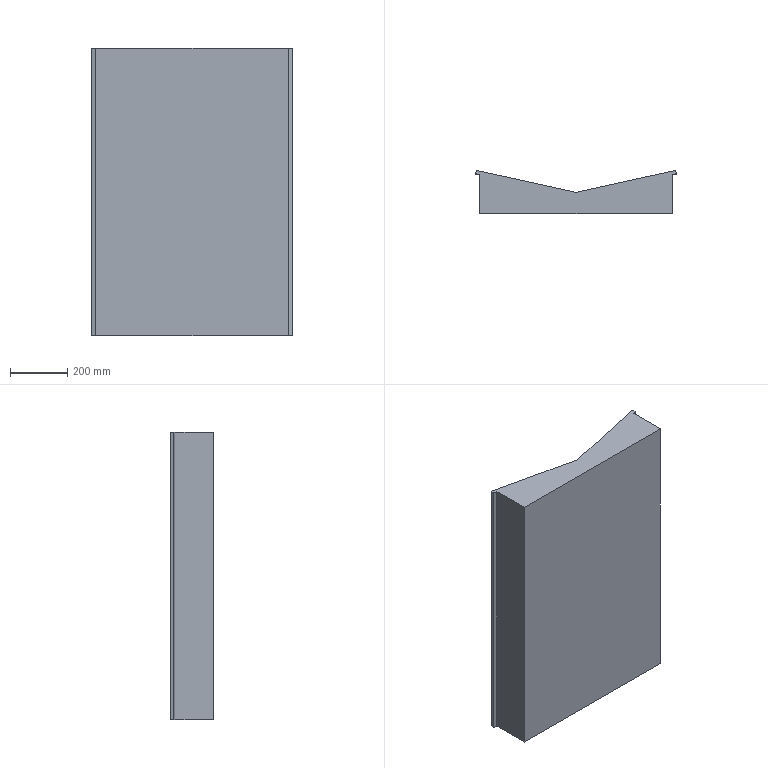Part | SolidWorks | features BaseBody 1 | 1 solid | 12 faces | box 698.157 x 148.827 x 1000 mm | volume 73538698 mm3 | plane 12
STEP:
#1=CARTESIAN_POINT('',(3335.082,1662.192,0.));
#2=VERTEX_POINT('',#1);
#3=CARTESIAN_POINT('',(3335.082,1796.192,0.));
#4=VERTEX_POINT('',#3);
#5=CARTESIAN_POINT('',(3335.082,0.,0.));
#6=DIRECTION('',(0.,1.,0.));
#7=VECTOR('',#6,1000.);
#8=LINE('',#5,#7);
#9=EDGE_CURVE('',#2,#4,#8,.T.);
#10=ORIENTED_EDGE('',*,*,#9,.T.);
#11=CARTESIAN_POINT('',(3335.082,1796.192,1000.));
#12=VERTEX_POINT('',#11);
#13=CARTESIAN_POINT('',(3335.082,1796.192,1000.));
#14=DIRECTION('',(0.,0.,-1.));
#15=VECTOR('',#14,1000.);
#16=LINE('',#13,#15);
#17=EDGE_CURVE('',#12,#4,#16,.T.);
#18=ORIENTED_EDGE('',*,*,#17,.F.);
#19=CARTESIAN_POINT('',(3335.082,1662.192,1000.));
#20=VERTEX_POINT('',#19);
#21=CARTESIAN_POINT('',(3335.082,0.,1000.));
#22=DIRECTION('',(0.,1.,0.));
#23=VECTOR('',#22,1000.);
#24=LINE('',#21,#23);
#25=EDGE_CURVE('',#20,#12,#24,.T.);
#26=ORIENTED_EDGE('',*,*,#25,.F.);
#27=CARTESIAN_POINT('',(3335.082,1662.192,1000.));
#28=DIRECTION('',(0.,0.,-1.));
#29=VECTOR('',#28,1000.);
#30=LINE('',#27,#29);
#31=EDGE_CURVE('',#20,#2,#30,.T.);
#32=ORIENTED_EDGE('',*,*,#31,.T.);
#33=EDGE_LOOP('',(#10,#18,#26,#32));
#34=FACE_OUTER_BOUND('',#33,.T.);
#35=CARTESIAN_POINT('',(3335.082,0.,1000.));
#36=DIRECTION('',(-1.,0.,0.));
#37=DIRECTION('',(0.,0.,1.));
#38=AXIS2_PLACEMENT_3D('',#35,#36,#37);
#39=PLANE('',#38);
#40=ADVANCED_FACE('',(#34),#39,.F.);
#41=CARTESIAN_POINT('',(3349.16,1799.302,0.));
#42=VERTEX_POINT('',#41);
#43=CARTESIAN_POINT('',(-223.148,1010.195,0.));
#44=DIRECTION('',(-0.9765,-0.2157,0.));
#45=VECTOR('',#44,1000.);
#46=LINE('',#43,#45);
#47=EDGE_CURVE('',#42,#4,#46,.T.);
#48=ORIENTED_EDGE('',*,*,#47,.F.);
#49=CARTESIAN_POINT('',(3349.16,1799.302,1000.));
#50=VERTEX_POINT('',#49);
#51=CARTESIAN_POINT('',(3349.16,1799.302,1000.));
#52=DIRECTION('',(0.,0.,-1.));
#53=VECTOR('',#52,1000.);
#54=LINE('',#51,#53);
#55=EDGE_CURVE('',#50,#42,#54,.T.);
#56=ORIENTED_EDGE('',*,*,#55,.F.);
#57=CARTESIAN_POINT('',(-223.148,1010.195,1000.));
#58=DIRECTION('',(-0.9765,-0.2157,0.));
#59=VECTOR('',#58,1000.);
#60=LINE('',#57,#59);
#61=EDGE_CURVE('',#50,#12,#60,.T.);
#62=ORIENTED_EDGE('',*,*,#61,.T.);
#63=ORIENTED_EDGE('',*,*,#17,.T.);
#64=EDGE_LOOP('',(#48,#56,#62,#63));
#65=FACE_OUTER_BOUND('',#64,.T.);
#66=CARTESIAN_POINT('',(-223.148,1010.195,1000.));
#67=DIRECTION('',(0.2157,-0.9765,0.));
#68=DIRECTION('',(0.9765,0.2157,0.));
#69=AXIS2_PLACEMENT_3D('',#66,#67,#68);
#70=PLANE('',#69);
#71=ADVANCED_FACE('',(#65),#70,.T.);
#72=CARTESIAN_POINT('',(3346.572,1811.019,0.));
#73=VERTEX_POINT('',#72);
#74=CARTESIAN_POINT('',(3572.308,789.107,0.));
#75=DIRECTION('',(0.2157,-0.9765,0.));
#76=VECTOR('',#75,1000.);
#77=LINE('',#74,#76);
#78=EDGE_CURVE('',#73,#42,#77,.T.);
#79=ORIENTED_EDGE('',*,*,#78,.F.);
#80=CARTESIAN_POINT('',(3346.572,1811.019,1000.));
#81=VERTEX_POINT('',#80);
#82=CARTESIAN_POINT('',(3346.572,1811.019,1000.));
#83=DIRECTION('',(0.,0.,-1.));
#84=VECTOR('',#83,1000.);
#85=LINE('',#82,#84);
#86=EDGE_CURVE('',#81,#73,#85,.T.);
#87=ORIENTED_EDGE('',*,*,#86,.F.);
#88=CARTESIAN_POINT('',(3572.308,789.107,1000.));
#89=DIRECTION('',(0.2157,-0.9765,0.));
#90=VECTOR('',#89,1000.);
#91=LINE('',#88,#90);
#92=EDGE_CURVE('',#81,#50,#91,.T.);
#93=ORIENTED_EDGE('',*,*,#92,.T.);
#94=ORIENTED_EDGE('',*,*,#55,.T.);
#95=EDGE_LOOP('',(#79,#87,#93,#94));
#96=FACE_OUTER_BOUND('',#95,.T.);
#97=CARTESIAN_POINT('',(3572.308,789.107,1000.));
#98=DIRECTION('',(0.9765,0.2157,0.));
#99=DIRECTION('',(-0.2157,0.9765,0.));
#100=AXIS2_PLACEMENT_3D('',#97,#98,#99);
#101=PLANE('',#100);
#102=ADVANCED_FACE('',(#96),#101,.T.);
#103=CARTESIAN_POINT('',(3001.807,1734.862,0.));
#104=VERTEX_POINT('',#103);
#105=CARTESIAN_POINT('',(-225.736,1021.913,0.));
#106=DIRECTION('',(-0.9765,-0.2157,0.));
#107=VECTOR('',#106,1000.);
#108=LINE('',#105,#107);
#109=EDGE_CURVE('',#73,#104,#108,.T.);
#110=ORIENTED_EDGE('',*,*,#109,.T.);
#111=CARTESIAN_POINT('',(3001.807,1734.862,1000.));
#112=VERTEX_POINT('',#111);
#113=CARTESIAN_POINT('',(3001.807,1734.862,1000.));
#114=DIRECTION('',(0.,0.,-1.));
#115=VECTOR('',#114,1000.);
#116=LINE('',#113,#115);
#117=EDGE_CURVE('',#112,#104,#116,.T.);
#118=ORIENTED_EDGE('',*,*,#117,.F.);
#119=CARTESIAN_POINT('',(-225.736,1021.913,1000.));
#120=DIRECTION('',(-0.9765,-0.2157,0.));
#121=VECTOR('',#120,1000.);
#122=LINE('',#119,#121);
#123=EDGE_CURVE('',#81,#112,#122,.T.);
#124=ORIENTED_EDGE('',*,*,#123,.F.);
#125=ORIENTED_EDGE('',*,*,#86,.T.);
#126=EDGE_LOOP('',(#110,#118,#124,#125));
#127=FACE_OUTER_BOUND('',#126,.T.);
#128=CARTESIAN_POINT('',(-225.736,1021.913,1000.));
#129=DIRECTION('',(0.2157,-0.9765,0.));
#130=DIRECTION('',(0.9765,0.2157,0.));
#131=AXIS2_PLACEMENT_3D('',#128,#129,#130);
#132=PLANE('',#131);
#133=ADVANCED_FACE('',(#127),#132,.F.);
#134=CARTESIAN_POINT('',(2998.356,1734.862,0.));
#135=VERTEX_POINT('',#134);
#136=CARTESIAN_POINT('',(0.,1734.862,0.));
#137=DIRECTION('',(-1.,0.,0.));
#138=VECTOR('',#137,1000.);
#139=LINE('',#136,#138);
#140=EDGE_CURVE('',#104,#135,#139,.T.);
#141=ORIENTED_EDGE('',*,*,#140,.T.);
#142=CARTESIAN_POINT('',(2998.356,1734.862,1000.));
#143=VERTEX_POINT('',#142);
#144=CARTESIAN_POINT('',(2998.356,1734.862,1000.));
#145=DIRECTION('',(0.,0.,-1.));
#146=VECTOR('',#145,1000.);
#147=LINE('',#144,#146);
#148=EDGE_CURVE('',#143,#135,#147,.T.);
#149=ORIENTED_EDGE('',*,*,#148,.F.);
#150=CARTESIAN_POINT('',(0.,1734.862,1000.));
#151=DIRECTION('',(-1.,0.,0.));
#152=VECTOR('',#151,1000.);
#153=LINE('',#150,#152);
#154=EDGE_CURVE('',#112,#143,#153,.T.);
#155=ORIENTED_EDGE('',*,*,#154,.F.);
#156=ORIENTED_EDGE('',*,*,#117,.T.);
#157=EDGE_LOOP('',(#141,#149,#155,#156));
#158=FACE_OUTER_BOUND('',#157,.T.);
#159=CARTESIAN_POINT('',(0.,1734.862,1000.));
#160=DIRECTION('',(0.,-1.,0.));
#161=DIRECTION('',(0.,0.,-1.));
#162=AXIS2_PLACEMENT_3D('',#159,#160,#161);
#163=PLANE('',#162);
#164=ADVANCED_FACE('',(#158),#163,.F.);
#165=CARTESIAN_POINT('',(2653.592,1811.019,0.));
#166=VERTEX_POINT('',#165);
#167=CARTESIAN_POINT('',(504.892,2285.658,0.));
#168=DIRECTION('',(0.9765,-0.2157,0.));
#169=VECTOR('',#168,1000.);
#170=LINE('',#167,#169);
#171=EDGE_CURVE('',#166,#135,#170,.T.);
#172=ORIENTED_EDGE('',*,*,#171,.F.);
#173=CARTESIAN_POINT('',(2653.592,1811.019,1000.));
#174=VERTEX_POINT('',#173);
#175=CARTESIAN_POINT('',(2653.592,1811.019,1000.));
#176=DIRECTION('',(0.,0.,-1.));
#177=VECTOR('',#176,1000.);
#178=LINE('',#175,#177);
#179=EDGE_CURVE('',#174,#166,#178,.T.);
#180=ORIENTED_EDGE('',*,*,#179,.F.);
#181=CARTESIAN_POINT('',(504.892,2285.658,1000.));
#182=DIRECTION('',(0.9765,-0.2157,0.));
#183=VECTOR('',#182,1000.);
#184=LINE('',#181,#183);
#185=EDGE_CURVE('',#174,#143,#184,.T.);
#186=ORIENTED_EDGE('',*,*,#185,.T.);
#187=ORIENTED_EDGE('',*,*,#148,.T.);
#188=EDGE_LOOP('',(#172,#180,#186,#187));
#189=FACE_OUTER_BOUND('',#188,.T.);
#190=CARTESIAN_POINT('',(504.892,2285.658,1000.));
#191=DIRECTION('',(0.2157,0.9765,0.));
#192=DIRECTION('',(-0.9765,0.2157,0.));
#193=AXIS2_PLACEMENT_3D('',#190,#191,#192);
#194=PLANE('',#193);
#195=ADVANCED_FACE('',(#189),#194,.T.);
#196=CARTESIAN_POINT('',(2651.003,1799.302,0.));
#197=VERTEX_POINT('',#196);
#198=CARTESIAN_POINT('',(2148.7,-474.638,0.));
#199=DIRECTION('',(-0.2157,-0.9765,0.));
#200=VECTOR('',#199,1000.);
#201=LINE('',#198,#200);
#202=EDGE_CURVE('',#166,#197,#201,.T.);
#203=ORIENTED_EDGE('',*,*,#202,.T.);
#204=CARTESIAN_POINT('',(2651.003,1799.302,1000.));
#205=VERTEX_POINT('',#204);
#206=CARTESIAN_POINT('',(2651.003,1799.302,1000.));
#207=DIRECTION('',(0.,0.,-1.));
#208=VECTOR('',#207,1000.);
#209=LINE('',#206,#208);
#210=EDGE_CURVE('',#205,#197,#209,.T.);
#211=ORIENTED_EDGE('',*,*,#210,.F.);
#212=CARTESIAN_POINT('',(2148.7,-474.638,1000.));
#213=DIRECTION('',(-0.2157,-0.9765,0.));
#214=VECTOR('',#213,1000.);
#215=LINE('',#212,#214);
#216=EDGE_CURVE('',#174,#205,#215,.T.);
#217=ORIENTED_EDGE('',*,*,#216,.F.);
#218=ORIENTED_EDGE('',*,*,#179,.T.);
#219=EDGE_LOOP('',(#203,#211,#217,#218));
#220=FACE_OUTER_BOUND('',#219,.T.);
#221=CARTESIAN_POINT('',(2148.7,-474.638,1000.));
#222=DIRECTION('',(0.9765,-0.2157,0.));
#223=DIRECTION('',(0.2157,0.9765,0.));
#224=AXIS2_PLACEMENT_3D('',#221,#222,#223);
#225=PLANE('',#224);
#226=ADVANCED_FACE('',(#220),#225,.F.);
#227=CARTESIAN_POINT('',(2665.082,1796.192,0.));
#228=VERTEX_POINT('',#227);
#229=CARTESIAN_POINT('',(502.303,2273.94,0.));
#230=DIRECTION('',(0.9765,-0.2157,0.));
#231=VECTOR('',#230,1000.);
#232=LINE('',#229,#231);
#233=EDGE_CURVE('',#197,#228,#232,.T.);
#234=ORIENTED_EDGE('',*,*,#233,.T.);
#235=CARTESIAN_POINT('',(2665.082,1796.192,1000.));
#236=VERTEX_POINT('',#235);
#237=CARTESIAN_POINT('',(2665.082,1796.192,1000.));
#238=DIRECTION('',(0.,0.,-1.));
#239=VECTOR('',#238,1000.);
#240=LINE('',#237,#239);
#241=EDGE_CURVE('',#236,#228,#240,.T.);
#242=ORIENTED_EDGE('',*,*,#241,.F.);
#243=CARTESIAN_POINT('',(502.303,2273.94,1000.));
#244=DIRECTION('',(0.9765,-0.2157,0.));
#245=VECTOR('',#244,1000.);
#246=LINE('',#243,#245);
#247=EDGE_CURVE('',#205,#236,#246,.T.);
#248=ORIENTED_EDGE('',*,*,#247,.F.);
#249=ORIENTED_EDGE('',*,*,#210,.T.);
#250=EDGE_LOOP('',(#234,#242,#248,#249));
#251=FACE_OUTER_BOUND('',#250,.T.);
#252=CARTESIAN_POINT('',(502.303,2273.94,1000.));
#253=DIRECTION('',(0.2157,0.9765,0.));
#254=DIRECTION('',(-0.9765,0.2157,0.));
#255=AXIS2_PLACEMENT_3D('',#252,#253,#254);
#256=PLANE('',#255);
#257=ADVANCED_FACE('',(#251),#256,.F.);
#258=CARTESIAN_POINT('',(2665.082,1662.192,0.));
#259=VERTEX_POINT('',#258);
#260=CARTESIAN_POINT('',(2665.082,0.,0.));
#261=DIRECTION('',(0.,1.,0.));
#262=VECTOR('',#261,1000.);
#263=LINE('',#260,#262);
#264=EDGE_CURVE('',#259,#228,#263,.T.);
#265=ORIENTED_EDGE('',*,*,#264,.F.);
#266=CARTESIAN_POINT('',(2665.082,1662.192,1000.));
#267=VERTEX_POINT('',#266);
#268=CARTESIAN_POINT('',(2665.082,1662.192,1000.));
#269=DIRECTION('',(0.,0.,-1.));
#270=VECTOR('',#269,1000.);
#271=LINE('',#268,#270);
#272=EDGE_CURVE('',#267,#259,#271,.T.);
#273=ORIENTED_EDGE('',*,*,#272,.F.);
#274=CARTESIAN_POINT('',(2665.082,0.,1000.));
#275=DIRECTION('',(0.,1.,0.));
#276=VECTOR('',#275,1000.);
#277=LINE('',#274,#276);
#278=EDGE_CURVE('',#267,#236,#277,.T.);
#279=ORIENTED_EDGE('',*,*,#278,.T.);
#280=ORIENTED_EDGE('',*,*,#241,.T.);
#281=EDGE_LOOP('',(#265,#273,#279,#280));
#282=FACE_OUTER_BOUND('',#281,.T.);
#283=CARTESIAN_POINT('',(2665.082,0.,1000.));
#284=DIRECTION('',(-1.,0.,0.));
#285=DIRECTION('',(0.,-1.,0.));
#286=AXIS2_PLACEMENT_3D('',#283,#284,#285);
#287=PLANE('',#286);
#288=ADVANCED_FACE('',(#282),#287,.T.);
#289=CARTESIAN_POINT('',(0.,1662.192,0.));
#290=DIRECTION('',(1.,0.,0.));
#291=VECTOR('',#290,1000.);
#292=LINE('',#289,#291);
#293=EDGE_CURVE('',#259,#2,#292,.T.);
#294=ORIENTED_EDGE('',*,*,#293,.T.);
#295=ORIENTED_EDGE('',*,*,#31,.F.);
#296=CARTESIAN_POINT('',(0.,1662.192,1000.));
#297=DIRECTION('',(1.,0.,0.));
#298=VECTOR('',#297,1000.);
#299=LINE('',#296,#298);
#300=EDGE_CURVE('',#267,#20,#299,.T.);
#301=ORIENTED_EDGE('',*,*,#300,.F.);
#302=ORIENTED_EDGE('',*,*,#272,.T.);
#303=EDGE_LOOP('',(#294,#295,#301,#302));
#304=FACE_OUTER_BOUND('',#303,.T.);
#305=CARTESIAN_POINT('',(0.,1662.192,1000.));
#306=DIRECTION('',(0.,1.,0.));
#307=DIRECTION('',(0.,0.,1.));
#308=AXIS2_PLACEMENT_3D('',#305,#306,#307);
#309=PLANE('',#308);
#310=ADVANCED_FACE('',(#304),#309,.F.);
#311=ORIENTED_EDGE('',*,*,#25,.T.);
#312=ORIENTED_EDGE('',*,*,#61,.F.);
#313=ORIENTED_EDGE('',*,*,#92,.F.);
#314=ORIENTED_EDGE('',*,*,#123,.T.);
#315=ORIENTED_EDGE('',*,*,#154,.T.);
#316=ORIENTED_EDGE('',*,*,#185,.F.);
#317=ORIENTED_EDGE('',*,*,#216,.T.);
#318=ORIENTED_EDGE('',*,*,#247,.T.);
#319=ORIENTED_EDGE('',*,*,#278,.F.);
#320=ORIENTED_EDGE('',*,*,#300,.T.);
#321=EDGE_LOOP('',(#311,#312,#313,#314,#315,#316,#317,#318,#319,#320));
#322=FACE_OUTER_BOUND('',#321,.T.);
#323=CARTESIAN_POINT('',(0.,0.,1000.));
#324=DIRECTION('',(0.,0.,1.));
#325=DIRECTION('',(1.,0.,0.));
#326=AXIS2_PLACEMENT_3D('',#323,#324,#325);
#327=PLANE('',#326);
#328=ADVANCED_FACE('',(#322),#327,.T.);
#329=ORIENTED_EDGE('',*,*,#9,.F.);
#330=ORIENTED_EDGE('',*,*,#293,.F.);
#331=ORIENTED_EDGE('',*,*,#264,.T.);
#332=ORIENTED_EDGE('',*,*,#233,.F.);
#333=ORIENTED_EDGE('',*,*,#202,.F.);
#334=ORIENTED_EDGE('',*,*,#171,.T.);
#335=ORIENTED_EDGE('',*,*,#140,.F.);
#336=ORIENTED_EDGE('',*,*,#109,.F.);
#337=ORIENTED_EDGE('',*,*,#78,.T.);
#338=ORIENTED_EDGE('',*,*,#47,.T.);
#339=EDGE_LOOP('',(#329,#330,#331,#332,#333,#334,#335,#336,#337,#338));
#340=FACE_OUTER_BOUND('',#339,.T.);
#341=CARTESIAN_POINT('',(0.,0.,0.));
#342=DIRECTION('',(0.,0.,1.));
#343=DIRECTION('',(1.,0.,0.));
#344=AXIS2_PLACEMENT_3D('',#341,#342,#343);
#345=PLANE('',#344);
#346=ADVANCED_FACE('',(#340),#345,.F.);
#347=CLOSED_SHELL('',(#40,#71,#102,#133,#164,#195,#226,#257,#288,#310,#328,#346));
#348=MANIFOLD_SOLID_BREP('',#347);
#349=CARTESIAN_POINT('',(0.,0.,0.));
#350=DIRECTION('',(0.,0.,1.));
#351=DIRECTION('',(1.,0.,0.));
#352=AXIS2_PLACEMENT_3D('',#349,#350,#351);
#353=(LENGTH_UNIT()NAMED_UNIT(*)SI_UNIT(.MILLI.,.METRE.));
#354=UNCERTAINTY_MEASURE_WITH_UNIT(LENGTH_MEASURE(0.00001),#353,'','');
#355=(NAMED_UNIT(*)PLANE_ANGLE_UNIT()SI_UNIT($,.RADIAN.));
#356=(NAMED_UNIT(*)SI_UNIT($,.STERADIAN.)SOLID_ANGLE_UNIT());
#357=(GEOMETRIC_REPRESENTATION_CONTEXT(3)GLOBAL_UNCERTAINTY_ASSIGNED_CONTEXT((#354))GLOBAL_UNIT_ASSIGNED_CONTEXT((#353,#355,#356))REPRESENTATION_CONTEXT('',''));
#358=ADVANCED_BREP_SHAPE_REPRESENTATION('',(#348,#352),#357);